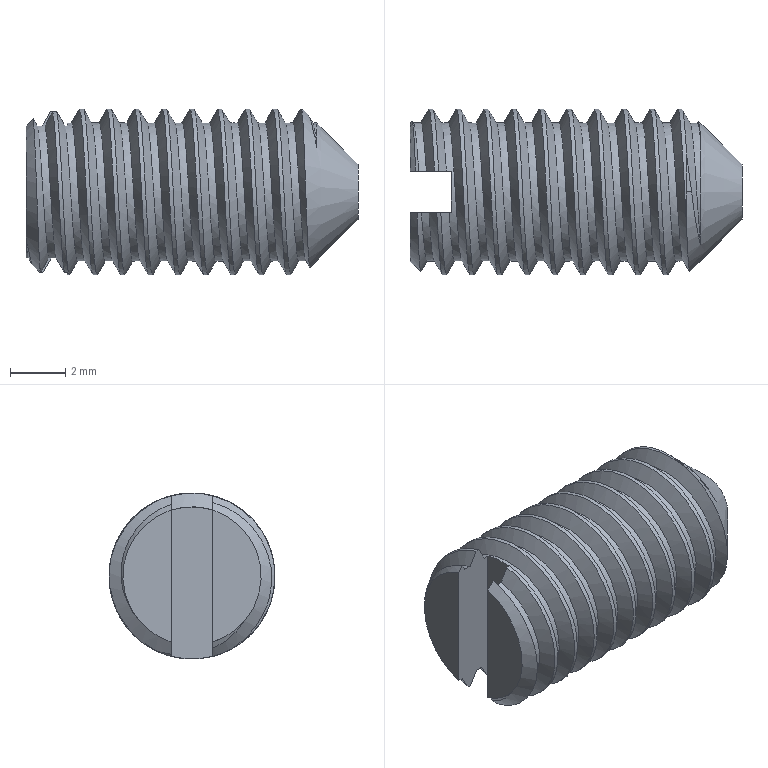Part | NX | features DATUM_CSYS 3, SKETCH 2, CHAMFER 1, EXTRUDE 1, SWP104 1, THREADS 1 | 1 solid | 26 faces | box 12 x 6 x 6 mm | volume 246.547 mm3 | spline 8 | cylinder 7 | plane 6 | cone 5 | commonest cylinder face diameters 5 x4 6 x3